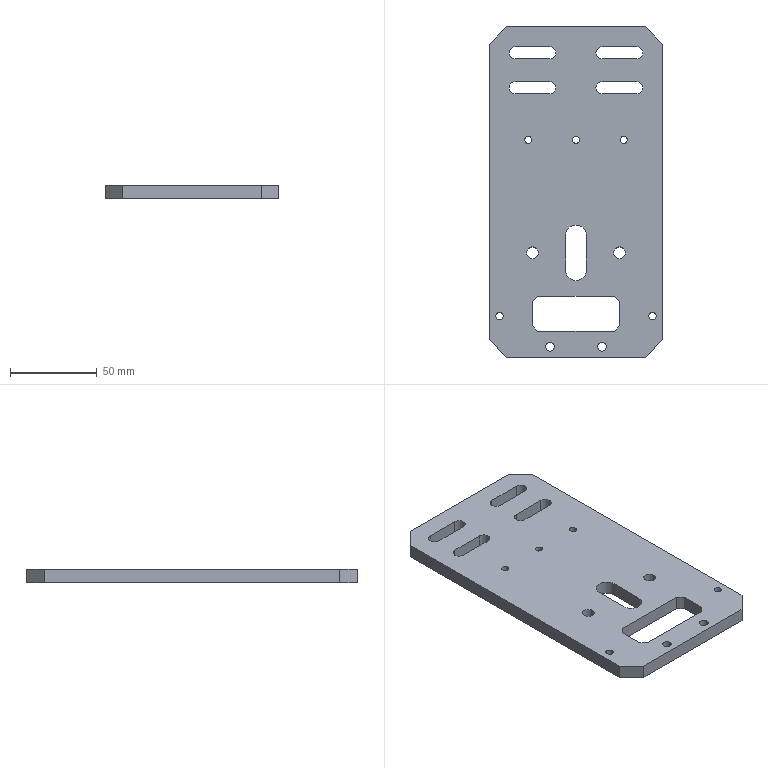Part | SolidWorks | features 3DProfileFeature 2, HoleWzd 2, Chamfer 1, Extrusion 1, ICE 1, LPattern 1 | 1 solid | 60 faces | box 100 x 190 x 8 mm | volume 132589 mm3 | cylinder 32 | plane 28 | commonest cylinder face diameters 7 x12 4 x6 4.2 x4 5 x4 6.8 x4 12 x2